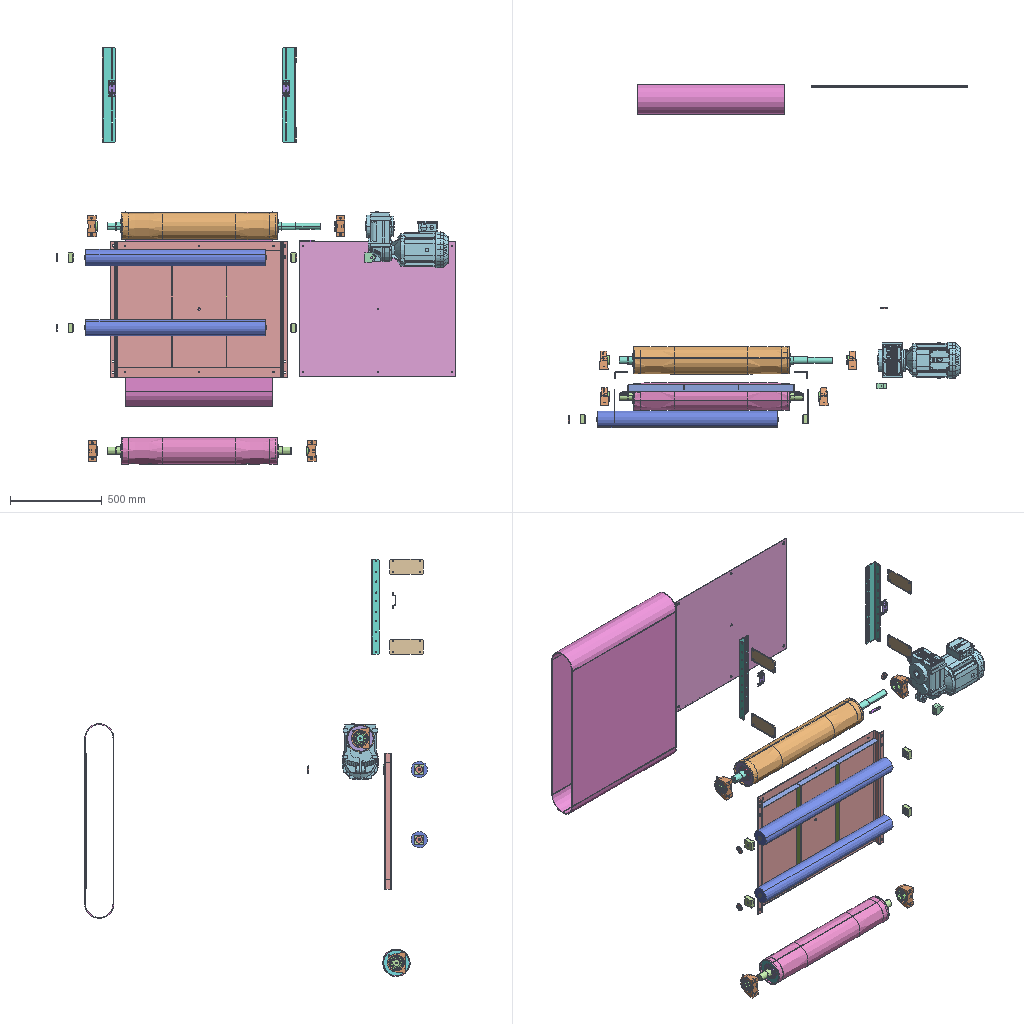Assembly | SolidWorks | 37 different items | 103 placed | box 2175 x 1865 x 2269 mm
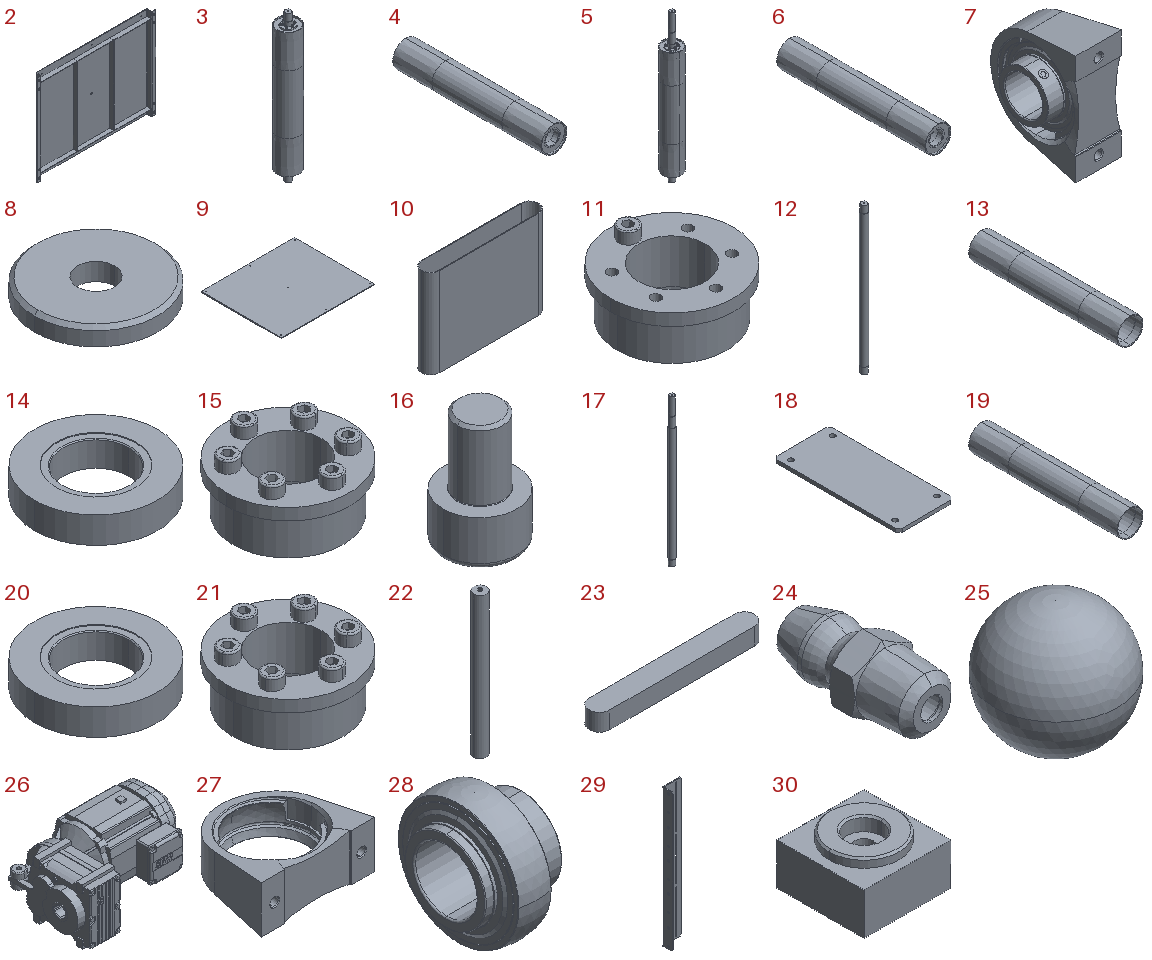Parts list (item | name | quantity | parent item | size | volume | features):
1 | XX8D684 | x1 | - | - | - | -
2 | (subassembly) | x1 | - | 966 x 43 x 740 mm | 2615508 mm3 | -
3 | (subassembly) | x1 | - | 150 x 150 x 1000 mm | 4622991 mm3 | -
4 | (subassembly) | x1 | - | 150 x 850 x 150 mm | 2873344 mm3 | features CompositeCurve 1
5 | (subassembly) | x1 | - | 150 x 150 x 1164 mm | 4781724 mm3 | -
6 | (subassembly) | x1 | - | 150 x 850 x 150 mm | 2873344 mm3 | features CompositeCurve 1
7 | (subassembly) | x4 | - | 54.2 x 99.5 x 116 mm | 238487 mm3 | features AEMSimFeature 1
8 | - | x1 | - | 35 x 35 x 5 mm | 4324 mm3 | features Chamfer 1, Extrusion 1
9 | - | x1 | - | 850 x 735 x 8 mm | 4972189 mm3 | features ICE 4, Chamfer 1, Extrusion 1
10 | - | x1 | - | 1060 x 160 x 800 mm | 9147787 mm3 | features ExtruThin 1
11 | - | x1 | - | 84 x 84 x 41 mm | 89359 mm3 | features BaseBody 3, ICE 1
12 | - | x1 | in 3 | 45 x 45 x 1000 mm | 1555641 mm3 | features HoleWzd 2, ICE 2, Chamfer 1, Extrusion 1, Fillet 1
13 | - | x1 | in 3 | 150 x 850 x 150 mm | 2218913 mm3 | features ICE 3, Chamfer 1, Revolution 1
14 | - | x2 | in 3 | 140 x 140 x 30 mm | 327215 mm3 | features Chamfer 1, Extrusion 1, ICE 1
15 | - | x2 | in 3 | 84 x 84 x 41 mm | 97003 mm3 | features BaseBody 8
16 | - | x1 | - | 13 x 13 x 20 mm | 1529 mm3 | features Fillet 2, ICE 2, Chamfer 1, Extrusion 1
17 | - | x1 | in 5 | 45 x 45 x 1164 mm | 1714375 mm3 | features ICE 4, Chamfer 2, HoleWzd 2, Extrusion 1, Fillet 1
18 | - | x4 | - | 80 x 180 x 5 mm | 70980 mm3 | features Chamfer 1, Extrusion 1, ICE 1
19 | - | x1 | in 5 | 150 x 850 x 150 mm | 2218913 mm3 | features ICE 3, Chamfer 1, Revolution 1
20 | - | x2 | in 5 | 140 x 140 x 30 mm | 327215 mm3 | features Chamfer 1, Extrusion 1, ICE 1
21 | - | x2 | in 5 | 84 x 84 x 41 mm | 97003 mm3 | features BaseBody 8
22 | - | x2 | - | 89 x 89 x 992 mm | 5903477 mm3 | features ICE 3, HoleWzd 2, Extrusion 1
23 | - | x1 | - | 80 x 10 x 8.3 mm | 6462 mm3 | features Extrusion 1
24 | - | x4 | in 7 | 7.001 x 16.4 x 8.083 mm | 360.824 mm3 | features BaseBody 1
25 | - | x36 | in 7 | 12.303 x 12.303 x 12.303 mm | 975.061 mm3 | features BaseBody 1
26 | - | x1 | - | 447.5 x 307.56 x 199 mm | 13556932 mm3 | features MBimport 1
27 | - | x4 | in 7 | 116 x 99.5 x 48 mm | 160162 mm3 | features BaseBody 1
28 | - | x4 | in 7 | 49.2 x 80 x 80 mm | 69188 mm3 | features BaseBody 1
29 | - | x2 | - | 70 x 40 x 515 mm | 153119 mm3 | features ICE 2, Chamfer 1, Extrusion 1
30 | - | x4 | - | 50 x 50 x 29 mm | 61857 mm3 | features ICE 3, Chamfer 2, Extrusion 1
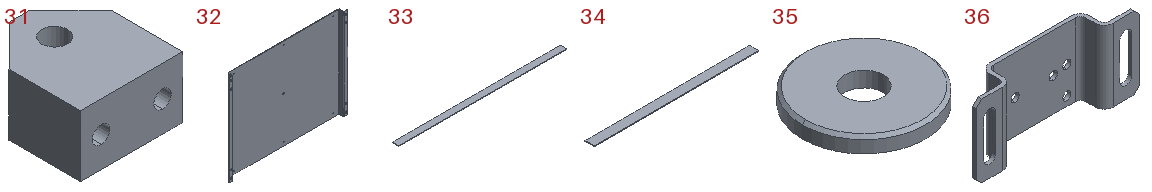31 | - | x1 | - | 50 x 55 x 30 mm | 63941 mm3 | features Chamfer 1, Extrusion 1, HoleWzd 1, ICE 1
32 | - | x1 | in 2 | 966 x 43 x 740 mm | 2293433 mm3 | features ICE 3, Extrusion 1
33 | - | x2 | in 2 | 900 x 35 x 3 mm | 94468 mm3 | features Extrusion 1, Fillet 1
34 | - | x2 | in 2 | 634 x 35 x 3 mm | 66570 mm3 | features Extrusion 1
35 | - | x5 | - | 40 x 40 x 5 mm | 5608 mm3 | features Chamfer 1, Extrusion 1
36 | - | x2 | - | 90 x 15 x 40 mm | 7851 mm3 | features ICE 2, Chamfer 1, Extrusion 1
37 | FA47_GDRN100LS4_20250626_045713_7NP8w_c0xE_eIM1imQzl3g.stp | x1 | - | - | - | -
Mates (type | each side: item.copy, entity, surface, feature):
In the top assembly
Coincident | 32.1 face plane Boss-Extrude 1 | 9.1 face plane Boss-Extrude 1
Concentric | 32.1 edge | 9.1 edge | 2 times
Parallel | 32.1 face plane Boss-Extrude 1 | 14.1 face plane Boss-Extrude 1
Parallel | 32.1 face plane Boss-Extrude 1 | 20.1 face plane Boss-Extrude 1
Coincident | 20.1 face plane Boss-Extrude 1 | 14.2 face plane Boss-Extrude 1
DistanceDim | 13.1 face cylinder Revolve 1 | 19.1 face cylinder Revolve 1
Tangent | 9.1 face plane Boss-Extrude 1 | 13.1 face cylinder Revolve 1
Width | 14.2 face plane Boss-Extrude 1 | 14.1 face plane Boss-Extrude 1 | 32.1 face plane Boss-Extrude 1 | 32.1 face plane Boss-Extrude 1
Concentric | 12.1 face cylinder Boss-Extrude 3 | 28.1 face cylinder YAR 208-2F-51.810300220880-b(1)
Coincident | 12.1 face plane Boss-Extrude 1 | 28.1 face plane YAR 208-2F-51.810300220880-b(1)
Concentric | 12.1 face cylinder Boss-Extrude 2 | 28.2 face cylinder YAR 208-2F-51.810300220880-b(1)
Coincident | 12.1 face plane Boss-Extrude 1 | 28.2 face plane YAR 208-2F-51.810300220880-b(1)
Coincident | 27.1 face plane SYF 508 -h(1) | 27.2 face plane SYF 508 -h(1)
Parallel | 32.1 face plane Boss-Extrude 1 | 27.1 face plane SYF 508 -h(1)
Concentric | 17.1 face cylinder Boss-Extrude 2 | 28.3 face cylinder YAR 208-2F-51.810300220880-b(1)
Coincident | 17.1 face plane Boss-Extrude 1 | 28.3 face plane YAR 208-2F-51.810300220880-b(1)
Concentric | 17.1 face cylinder Boss-Extrude 4 | 28.4 face cylinder YAR 208-2F-51.810300220880-b(1)
Coincident | 17.1 face plane Boss-Extrude 1 | 28.4 face plane YAR 208-2F-51.810300220880-b(1)
Coincident | 27.3 face plane SYF 508 -h(1) | 27.4 face plane SYF 508 -h(1)
Parallel | 32.1 face plane Boss-Extrude 1 | 27.3 face plane SYF 508 -h(1)
Width | 27.2 face plane SYF 508 -h(1) | 27.4 face plane SYF 508 -h(1) | 33.1 face plane Boss-Extrude 1 | 33.2 face plane Boss-Extrude 1
Coincident | 27.2 face plane SYF 508 -h(1) | 27.4 face plane SYF 508 -h(1)
Concentric | 17.1 face cylinder Cut-Extrude 1 | 23.1 face cylinder Boss-Extrude 1 | 2 times
Coincident | 17.1 face plane Cut-Extrude 1 | 23.1 face plane Boss-Extrude 1
Parallel | 32.1 face plane Boss-Extrude 1 | 31.1 face plane Boss-Extrude 1
Concentric | 22.1 face cylinder Boss-Extrude 1 | 30.1 face cylinder Cut-Extrude 2
Concentric | 22.1 face cylinder M10 Tapped Hole 2 | 30.2 face cylinder Cut-Extrude 2
Coincident | 22.1 face plane Boss-Extrude 2 | 30.1 face plane Boss-Extrude 1
Coincident | 22.1 face plane Boss-Extrude 3 | 30.2 face plane Boss-Extrude 1
Coincident | 30.3 face plane Boss-Extrude 1 | 35.1 face plane Boss-Extrude 1
Coincident | 30.2 face plane Boss-Extrude 1 | 35.2 face plane Boss-Extrude 1
Concentric | 30.3 face cylinder Cut-Extrude 2 | 35.1 face cylinder Boss-Extrude 1
Concentric | 30.2 face cylinder Cut-Extrude 2 | 35.2 face cylinder Boss-Extrude 1
Coincident | 30.4 face plane Boss-Extrude 1 | 35.3 face plane Boss-Extrude 1
Concentric | 30.4 face cylinder Cut-Extrude 2 | 35.3 face cylinder Boss-Extrude 1
Coincident | 30.1 face plane Boss-Extrude 1 | 35.4 face plane Boss-Extrude 1
Concentric | 30.1 face cylinder Cut-Extrude 2 | 35.4 face cylinder Boss-Extrude 1
Concentric | 13.1 face cylinder Revolve 1 | 10.1 face cylinder Extrude-Thin Wall 1
Coincident | 9.1 face plane Boss-Extrude 1 | 10.1 face plane Extrude-Thin Wall 1
Width | 10.1 face plane Extrude-Thin Wall 1 | 10.1 face plane Extrude-Thin Wall 1 | 20.1 face plane Boss-Extrude 1 | 20.2 face plane Boss-Extrude 1
Parallel | 30.1 face plane Boss-Extrude 1 | 30.4 face plane Boss-Extrude 1
Coincident | 30.3 face plane Boss-Extrude 1 | 22.2 face plane Boss-Extrude 3
Concentric | 35.1 face cylinder Boss-Extrude 1 | 22.2 face cylinder M10 Tapped Hole 1
Coincident | 30.4 face plane Boss-Extrude 1 | 22.2 face plane Boss-Extrude 2
Concentric | 30.4 face cylinder Cut-Extrude 2 | 22.2 face cylinder Boss-Extrude 1
Parallel | 32.1 face plane Boss-Extrude 1 | 35.1 face plane Boss-Extrude 1
Parallel | 30.4 face plane Boss-Extrude 1 | assembly plane
Coincident | 30.1 face plane Boss-Extrude 1 | 30.4 face plane Boss-Extrude 1
DistanceDim | 22.1 face cylinder Boss-Extrude 1 | 22.2 face cylinder Boss-Extrude 1
Tangent | 22.1 face cylinder Boss-Extrude 1 | 10.1 face plane Extrude-Thin Wall 1
Coincident | 22.1 face plane Boss-Extrude 1 | 22.2 face plane Boss-Extrude 1
Width | 30.4 face plane Boss-Extrude 1 | 30.1 face plane Boss-Extrude 1 | 33.1 face plane Boss-Extrude 1 | 33.2 face plane Boss-Extrude 1
Coincident | 29.1 face plane Boss-Extrude 1 | 18.1 face plane Boss-Extrude 1
Coincident | 29.1 face plane Boss-Extrude 1 | 18.2 face plane Boss-Extrude 1
Concentric | 29.1 face cylinder Cut-Extrude 1 | 18.2 face cylinder Cut-Extrude 1 | 2 times
Concentric | 29.1 face cylinder Cut-Extrude 1 | 18.1 face cylinder Cut-Extrude 1 | 2 times
Coincident | 29.2 face plane Boss-Extrude 1 | 18.3 face plane Boss-Extrude 1
Concentric | 29.2 face cylinder Cut-Extrude 1 | 18.3 face cylinder Cut-Extrude 1 | 2 times
Coincident | 29.2 face plane Boss-Extrude 1 | 18.4 face plane Boss-Extrude 1
Concentric | 29.2 face cylinder Cut-Extrude 1 | 18.4 face cylinder Cut-Extrude 1 | 2 times
Coincident | 18.2 face plane Boss-Extrude 1 | 18.3 face plane Boss-Extrude 1
Coincident | 29.1 face plane Boss-Extrude 1 | 29.2 face plane Boss-Extrude 1
Coincident | 32.1 face plane Boss-Extrude 1 | 29.2 face plane Boss-Extrude 1
Coincident | 31.1 face plane Boss-Extrude 1 | 18.4 face plane Boss-Extrude 1 | 3 times
Coincident | 32.1 face plane Boss-Extrude 1 | 29.1 face plane Boss-Extrude 1
Coincident | 30.3 face plane Boss-Extrude 1 | 30.2 face plane Boss-Extrude 1
Parallel | 30.1 face plane Boss-Extrude 1 | 30.2 face plane Boss-Extrude 1
Coincident | 29.1 face plane Boss-Extrude 1 | 36.1 face plane Boss-Extrude 1 | 2 times
Parallel | 29.1 face plane Boss-Extrude 1 | 36.1 face plane Boss-Extrude 1
Lock | 29.1 select_type:0 | 36.1 select_type:0
Coincident | 29.2 face plane Boss-Extrude 1 | 36.2 face plane Boss-Extrude 1 | 2 times
Coincident | 36.1 face plane Boss-Extrude 1 | 36.2 face plane Boss-Extrude 1
Width | 22.2 face plane Boss-Extrude 1 | 22.2 face plane Boss-Extrude 1 | 32.1 face plane Boss-Extrude 1 | 32.1 face plane Boss-Extrude 1
In subassembly 2
Concentric | 32.2 face cylinder Boss-Extrude 1 | 33.3 face cylinder Fillet 1
Coincident | 32.2 face plane Boss-Extrude 1 | 33.3 face plane Boss-Extrude 1
Coincident | 32.2 face plane Boss-Extrude 1 | 33.4 face plane Boss-Extrude 1 | 2 times
DistanceDim | 33.4 face plane Boss-Extrude 1 | 32.2 face plane Boss-Extrude 1
DistanceDim | 33.3 face plane Boss-Extrude 1 | 32.2 face plane Boss-Extrude 1
Coincident | 34.1 face plane Boss-Extrude 1 | 33.3 face plane Boss-Extrude 1
Coincident | 32.2 face plane Boss-Extrude 1 | 34.1 face plane Boss-Extrude 1
Coincident | 34.2 face plane Boss-Extrude 1 | 33.3 face plane Boss-Extrude 1
Coincident | 32.2 face plane Boss-Extrude 1 | 34.2 face plane Boss-Extrude 1
DistanceDim | 34.1 face plane Boss-Extrude 1 | 32.2 face plane Boss-Extrude 1
DistanceDim | 34.2 face plane Boss-Extrude 1 | 32.2 face plane Boss-Extrude 1
In subassembly 5
Concentric | 19.2 face cylinder Cut-Extrude 1 | 20.3 face cylinder Boss-Extrude 1
Coincident | 19.2 face plane Cut-Extrude 1 | 20.3 face plane Boss-Extrude 1
Concentric | 17.2 face cylinder Boss-Extrude 1 | 20.3 face cylinder Boss-Extrude 1
Concentric | 20.3 face cylinder Boss-Extrude 1 | 21.1 face cylinder 045-075-1-solid3
Coincident | 20.3 face plane Cut-Extrude 1 | 21.1 face plane 045-075-1-solid2
Concentric | 19.2 face cylinder Cut-Extrude 2 | 20.4 face cylinder Boss-Extrude 1
Concentric | 20.4 face cylinder Boss-Extrude 1 | 21.2 face cylinder 045-075-1-solid3
Coincident | 20.4 face plane Cut-Extrude 1 | 21.2 face plane 045-075-1-solid2
Coincident | 19.2 face plane Cut-Extrude 2 | 20.4 face plane Boss-Extrude 1
DistanceDim | 19.2 face plane Revolve 1 | 17.2 face plane Boss-Extrude 3
In subassembly 3
Concentric | 12.2 face cylinder Boss-Extrude 1 | 13.2 face cylinder Cut-Extrude 3
Concentric | 13.2 face cone Revolve 1 | 15.1 face cylinder 045-075-1-solid3
Concentric | 13.2 face cone Revolve 1 | 14.3 face cylinder Boss-Extrude 1
Coincident | 13.2 face plane Cut-Extrude 2 | 14.3 face plane Boss-Extrude 1
Coincident | 14.3 face plane Cut-Extrude 1 | 15.1 face plane 045-075-1-solid2
Concentric | 13.2 face cylinder Cut-Extrude 1 | 14.4 face cylinder Boss-Extrude 1
Concentric | 14.4 face cylinder Boss-Extrude 1 | 15.2 face cylinder 045-075-1-solid3
Coincident | 13.2 face plane Cut-Extrude 1 | 14.4 face plane Boss-Extrude 1
Coincident | 14.4 face plane Cut-Extrude 1 | 15.2 face plane 045-075-1-solid2
DistanceDim | 12.2 face plane Boss-Extrude 3 | 13.2 face plane Revolve 1